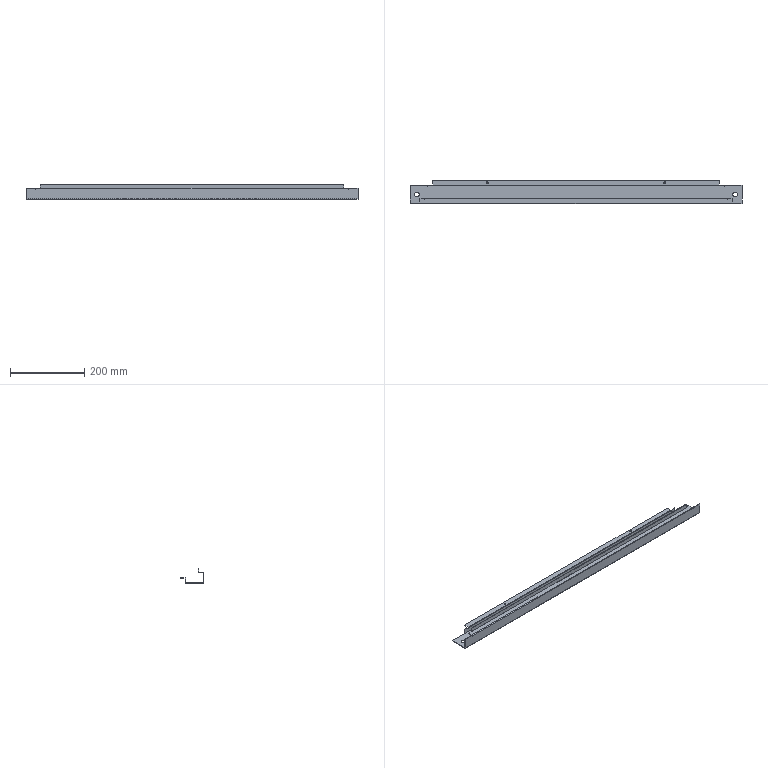Part | SolidWorks | features EdgeFlange 5, ICE 2, FlatPattern 1, SMBaseFlange 1, SheetMetal 1 | 1 solid | 86 faces | box 897 x 63.5 x 40.5 mm | volume 164762 mm3 | plane 68 | cylinder 18 | commonest cylinder face diameters 0.2 x5 3.2 x5 5.1 x4 13 x4